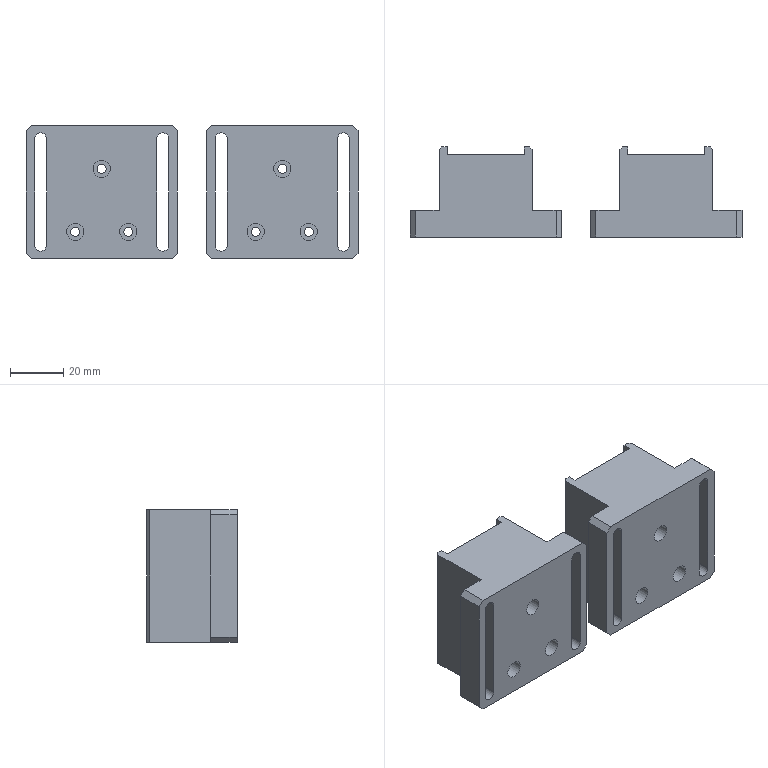Part | 2 solids | 74 faces | box 125 x 34 x 50 mm | volume 118900 mm3 | plane 54 | cylinder 20 | commonest cylinder face diameters 4.5 x8 3.4 x6 6.5 x6